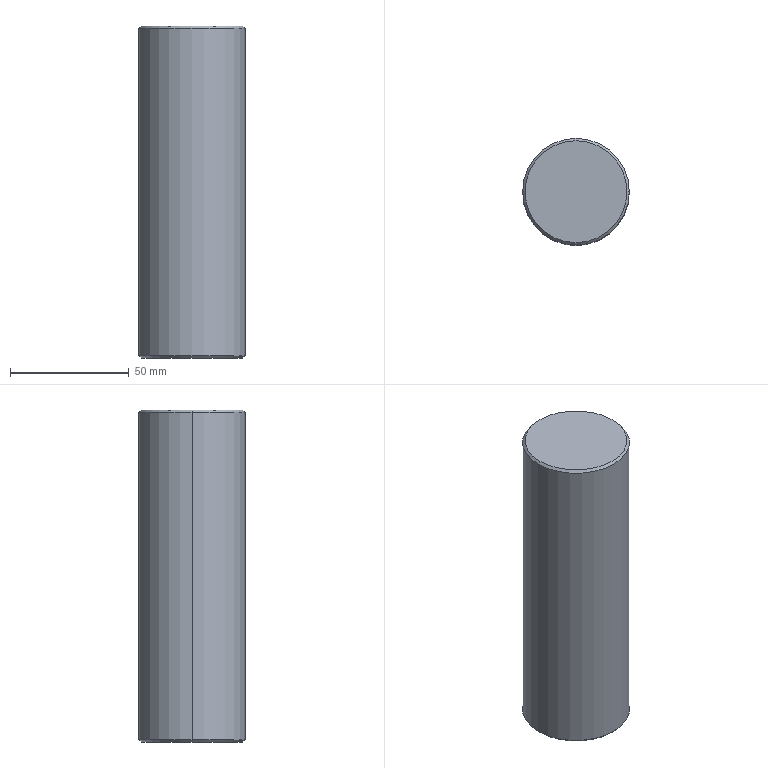Part | Creo | 1 solid | 16 faces | box 45 x 45 x 140 mm | volume 220997 mm3 | cone 8 | cylinder 6 | plane 2 | commonest cylinder face diameters 8.46 x2 10 x2 45 x2
STEP:
#1=CARTESIAN_POINT('',(0.,0.,0.));
#2=DIRECTION('',(0.,0.,1.));
#3=DIRECTION('',(1.,0.,0.));
#4=AXIS2_PLACEMENT_3D('',#1,#2,#3);
#5=CARTESIAN_POINT('',(-29.5,98.,-260.5));
#6=VERTEX_POINT('',#5);
#7=CARTESIAN_POINT('',(-72.5,98.,-260.5));
#8=VERTEX_POINT('',#7);
#9=CARTESIAN_POINT('',(-51.,98.,-260.5));
#10=DIRECTION('',(0.,0.,-1.));
#11=DIRECTION('',(1.,0.,0.));
#12=AXIS2_PLACEMENT_3D('',#9,#10,#11);
#13=CIRCLE('',#12,21.5);
#14=EDGE_CURVE('',#6,#8,#13,.T.);
#15=ORIENTED_EDGE('',*,*,#14,.F.);
#16=CARTESIAN_POINT('',(-51.,98.,-260.5));
#17=DIRECTION('',(0.,0.,-1.));
#18=DIRECTION('',(-1.,0.,0.));
#19=AXIS2_PLACEMENT_3D('',#16,#17,#18);
#20=CIRCLE('',#19,21.5);
#21=EDGE_CURVE('',#8,#6,#20,.T.);
#22=ORIENTED_EDGE('',*,*,#21,.F.);
#23=EDGE_LOOP('',(#15,#22));
#24=FACE_OUTER_BOUND('',#23,.F.);
#25=CARTESIAN_POINT('',(-56.,98.,-260.5));
#26=VERTEX_POINT('',#25);
#27=CARTESIAN_POINT('',(-46.,98.,-260.5));
#28=VERTEX_POINT('',#27);
#29=CARTESIAN_POINT('',(-51.,98.,-260.5));
#30=DIRECTION('',(0.,0.,1.));
#31=DIRECTION('',(-1.,0.,0.));
#32=AXIS2_PLACEMENT_3D('',#29,#30,#31);
#33=CIRCLE('',#32,5.);
#34=EDGE_CURVE('',#26,#28,#33,.T.);
#35=ORIENTED_EDGE('',*,*,#34,.F.);
#36=CARTESIAN_POINT('',(-51.,98.,-260.5));
#37=DIRECTION('',(0.,0.,1.));
#38=DIRECTION('',(1.,0.,0.));
#39=AXIS2_PLACEMENT_3D('',#36,#37,#38);
#40=CIRCLE('',#39,5.);
#41=EDGE_CURVE('',#28,#26,#40,.T.);
#42=ORIENTED_EDGE('',*,*,#41,.F.);
#43=EDGE_LOOP('',(#35,#42));
#44=FACE_BOUND('',#43,.F.);
#45=CARTESIAN_POINT('',(-51.,98.,-260.5));
#46=DIRECTION('',(0.,0.,1.));
#47=DIRECTION('',(1.,0.,0.));
#48=AXIS2_PLACEMENT_3D('',#45,#46,#47);
#49=PLANE('',#48);
#50=ADVANCED_FACE('',(#24,#44),#49,.F.);
#51=ORIENTED_EDGE('',*,*,#14,.T.);
#52=CARTESIAN_POINT('',(-73.5,98.,-259.5));
#53=VERTEX_POINT('',#52);
#54=CARTESIAN_POINT('',(-72.5,98.,-260.5));
#55=DIRECTION('',(-0.7071,0.,0.7071));
#56=VECTOR('',#55,1.414);
#57=LINE('',#54,#56);
#58=EDGE_CURVE('',#8,#53,#57,.T.);
#59=ORIENTED_EDGE('',*,*,#58,.T.);
#60=CARTESIAN_POINT('',(-28.5,98.,-259.5));
#61=VERTEX_POINT('',#60);
#62=CARTESIAN_POINT('',(-51.,98.,-259.5));
#63=DIRECTION('',(0.,0.,-1.));
#64=DIRECTION('',(1.,0.,0.));
#65=AXIS2_PLACEMENT_3D('',#62,#63,#64);
#66=CIRCLE('',#65,22.5);
#67=EDGE_CURVE('',#61,#53,#66,.T.);
#68=ORIENTED_EDGE('',*,*,#67,.F.);
#69=CARTESIAN_POINT('',(-29.5,98.,-260.5));
#70=DIRECTION('',(0.7071,0.,0.7071));
#71=VECTOR('',#70,1.414);
#72=LINE('',#69,#71);
#73=EDGE_CURVE('',#6,#61,#72,.T.);
#74=ORIENTED_EDGE('',*,*,#73,.F.);
#75=EDGE_LOOP('',(#51,#59,#68,#74));
#76=FACE_OUTER_BOUND('',#75,.F.);
#77=CARTESIAN_POINT('',(-51.,98.,-260.));
#78=DIRECTION('',(0.,0.,1.));
#79=DIRECTION('',(1.,0.,0.));
#80=AXIS2_PLACEMENT_3D('',#77,#78,#79);
#81=CONICAL_SURFACE('',#80,22.,45.);
#82=ADVANCED_FACE('',(#76),#81,.T.);
#83=ORIENTED_EDGE('',*,*,#21,.T.);
#84=ORIENTED_EDGE('',*,*,#73,.T.);
#85=CARTESIAN_POINT('',(-51.,98.,-259.5));
#86=DIRECTION('',(0.,0.,-1.));
#87=DIRECTION('',(-1.,0.,0.));
#88=AXIS2_PLACEMENT_3D('',#85,#86,#87);
#89=CIRCLE('',#88,22.5);
#90=EDGE_CURVE('',#53,#61,#89,.T.);
#91=ORIENTED_EDGE('',*,*,#90,.F.);
#92=ORIENTED_EDGE('',*,*,#58,.F.);
#93=EDGE_LOOP('',(#83,#84,#91,#92));
#94=FACE_OUTER_BOUND('',#93,.F.);
#95=CARTESIAN_POINT('',(-51.,98.,-260.));
#96=DIRECTION('',(0.,0.,1.));
#97=DIRECTION('',(1.,0.,0.));
#98=AXIS2_PLACEMENT_3D('',#95,#96,#97);
#99=CONICAL_SURFACE('',#98,22.,45.);
#100=ADVANCED_FACE('',(#94),#99,.T.);
#101=ORIENTED_EDGE('',*,*,#90,.T.);
#102=CARTESIAN_POINT('',(-28.5,98.,-121.5));
#103=VERTEX_POINT('',#102);
#104=CARTESIAN_POINT('',(-28.5,98.,-121.5));
#105=DIRECTION('',(0.,0.,-1.));
#106=VECTOR('',#105,138.);
#107=LINE('',#104,#106);
#108=EDGE_CURVE('',#103,#61,#107,.T.);
#109=ORIENTED_EDGE('',*,*,#108,.F.);
#110=CARTESIAN_POINT('',(-73.5,98.,-121.5));
#111=VERTEX_POINT('',#110);
#112=CARTESIAN_POINT('',(-51.,98.,-121.5));
#113=DIRECTION('',(0.,0.,1.));
#114=DIRECTION('',(1.,0.,0.));
#115=AXIS2_PLACEMENT_3D('',#112,#113,#114);
#116=CIRCLE('',#115,22.5);
#117=EDGE_CURVE('',#103,#111,#116,.T.);
#118=ORIENTED_EDGE('',*,*,#117,.T.);
#119=CARTESIAN_POINT('',(-73.5,98.,-121.5));
#120=DIRECTION('',(0.,0.,-1.));
#121=VECTOR('',#120,138.);
#122=LINE('',#119,#121);
#123=EDGE_CURVE('',#111,#53,#122,.T.);
#124=ORIENTED_EDGE('',*,*,#123,.T.);
#125=EDGE_LOOP('',(#101,#109,#118,#124));
#126=FACE_OUTER_BOUND('',#125,.F.);
#127=CARTESIAN_POINT('',(-51.,98.,-120.5));
#128=DIRECTION('',(0.,0.,-1.));
#129=DIRECTION('',(-1.,0.,0.));
#130=AXIS2_PLACEMENT_3D('',#127,#128,#129);
#131=CYLINDRICAL_SURFACE('',#130,22.5);
#132=ADVANCED_FACE('',(#126),#131,.T.);
#133=ORIENTED_EDGE('',*,*,#67,.T.);
#134=ORIENTED_EDGE('',*,*,#123,.F.);
#135=CARTESIAN_POINT('',(-51.,98.,-121.5));
#136=DIRECTION('',(0.,0.,1.));
#137=DIRECTION('',(-1.,0.,0.));
#138=AXIS2_PLACEMENT_3D('',#135,#136,#137);
#139=CIRCLE('',#138,22.5);
#140=EDGE_CURVE('',#111,#103,#139,.T.);
#141=ORIENTED_EDGE('',*,*,#140,.T.);
#142=ORIENTED_EDGE('',*,*,#108,.T.);
#143=EDGE_LOOP('',(#133,#134,#141,#142));
#144=FACE_OUTER_BOUND('',#143,.F.);
#145=CARTESIAN_POINT('',(-51.,98.,-120.5));
#146=DIRECTION('',(0.,0.,-1.));
#147=DIRECTION('',(-1.,0.,0.));
#148=AXIS2_PLACEMENT_3D('',#145,#146,#147);
#149=CYLINDRICAL_SURFACE('',#148,22.5);
#150=ADVANCED_FACE('',(#144),#149,.T.);
#151=ORIENTED_EDGE('',*,*,#140,.F.);
#152=CARTESIAN_POINT('',(-72.5,98.,-120.5));
#153=VERTEX_POINT('',#152);
#154=CARTESIAN_POINT('',(-72.5,98.,-120.5));
#155=DIRECTION('',(-0.7071,0.,-0.7071));
#156=VECTOR('',#155,1.414);
#157=LINE('',#154,#156);
#158=EDGE_CURVE('',#153,#111,#157,.T.);
#159=ORIENTED_EDGE('',*,*,#158,.F.);
#160=CARTESIAN_POINT('',(-29.5,98.,-120.5));
#161=VERTEX_POINT('',#160);
#162=CARTESIAN_POINT('',(-51.,98.,-120.5));
#163=DIRECTION('',(0.,0.,1.));
#164=DIRECTION('',(-1.,0.,0.));
#165=AXIS2_PLACEMENT_3D('',#162,#163,#164);
#166=CIRCLE('',#165,21.5);
#167=EDGE_CURVE('',#153,#161,#166,.T.);
#168=ORIENTED_EDGE('',*,*,#167,.T.);
#169=CARTESIAN_POINT('',(-29.5,98.,-120.5));
#170=DIRECTION('',(0.7071,0.,-0.7071));
#171=VECTOR('',#170,1.414);
#172=LINE('',#169,#171);
#173=EDGE_CURVE('',#161,#103,#172,.T.);
#174=ORIENTED_EDGE('',*,*,#173,.T.);
#175=EDGE_LOOP('',(#151,#159,#168,#174));
#176=FACE_OUTER_BOUND('',#175,.F.);
#177=CARTESIAN_POINT('',(-51.,98.,-121.));
#178=DIRECTION('',(0.,0.,-1.));
#179=DIRECTION('',(-1.,0.,0.));
#180=AXIS2_PLACEMENT_3D('',#177,#178,#179);
#181=CONICAL_SURFACE('',#180,22.,45.);
#182=ADVANCED_FACE('',(#176),#181,.T.);
#183=ORIENTED_EDGE('',*,*,#117,.F.);
#184=ORIENTED_EDGE('',*,*,#173,.F.);
#185=CARTESIAN_POINT('',(-51.,98.,-120.5));
#186=DIRECTION('',(0.,0.,1.));
#187=DIRECTION('',(1.,0.,0.));
#188=AXIS2_PLACEMENT_3D('',#185,#186,#187);
#189=CIRCLE('',#188,21.5);
#190=EDGE_CURVE('',#161,#153,#189,.T.);
#191=ORIENTED_EDGE('',*,*,#190,.T.);
#192=ORIENTED_EDGE('',*,*,#158,.T.);
#193=EDGE_LOOP('',(#183,#184,#191,#192));
#194=FACE_OUTER_BOUND('',#193,.F.);
#195=CARTESIAN_POINT('',(-51.,98.,-121.));
#196=DIRECTION('',(0.,0.,-1.));
#197=DIRECTION('',(-1.,0.,0.));
#198=AXIS2_PLACEMENT_3D('',#195,#196,#197);
#199=CONICAL_SURFACE('',#198,22.,45.);
#200=ADVANCED_FACE('',(#194),#199,.T.);
#201=ORIENTED_EDGE('',*,*,#190,.F.);
#202=ORIENTED_EDGE('',*,*,#167,.F.);
#203=EDGE_LOOP('',(#201,#202));
#204=FACE_OUTER_BOUND('',#203,.F.);
#205=CARTESIAN_POINT('',(-51.,98.,-120.5));
#206=DIRECTION('',(0.,0.,1.));
#207=DIRECTION('',(1.,0.,0.));
#208=AXIS2_PLACEMENT_3D('',#205,#206,#207);
#209=PLANE('',#208);
#210=ADVANCED_FACE('',(#204),#209,.T.);
#211=CARTESIAN_POINT('',(-46.,98.,-244.5));
#212=VERTEX_POINT('',#211);
#213=CARTESIAN_POINT('',(-56.,98.,-244.5));
#214=VERTEX_POINT('',#213);
#215=CARTESIAN_POINT('',(-51.,98.,-244.5));
#216=DIRECTION('',(0.,0.,-1.));
#217=DIRECTION('',(1.,0.,0.));
#218=AXIS2_PLACEMENT_3D('',#215,#216,#217);
#219=CIRCLE('',#218,5.);
#220=EDGE_CURVE('',#212,#214,#219,.T.);
#221=ORIENTED_EDGE('',*,*,#220,.T.);
#222=CARTESIAN_POINT('',(-56.,98.,-244.5));
#223=DIRECTION('',(0.,0.,-1.));
#224=VECTOR('',#223,16.);
#225=LINE('',#222,#224);
#226=EDGE_CURVE('',#214,#26,#225,.T.);
#227=ORIENTED_EDGE('',*,*,#226,.T.);
#228=ORIENTED_EDGE('',*,*,#34,.T.);
#229=CARTESIAN_POINT('',(-46.,98.,-244.5));
#230=DIRECTION('',(0.,0.,-1.));
#231=VECTOR('',#230,16.);
#232=LINE('',#229,#231);
#233=EDGE_CURVE('',#212,#28,#232,.T.);
#234=ORIENTED_EDGE('',*,*,#233,.F.);
#235=EDGE_LOOP('',(#221,#227,#228,#234));
#236=FACE_OUTER_BOUND('',#235,.F.);
#237=CARTESIAN_POINT('',(-51.,98.,-295.5));
#238=DIRECTION('',(0.,0.,-1.));
#239=DIRECTION('',(-1.,0.,0.));
#240=AXIS2_PLACEMENT_3D('',#237,#238,#239);
#241=CYLINDRICAL_SURFACE('',#240,5.);
#242=ADVANCED_FACE('',(#236),#241,.F.);
#243=CARTESIAN_POINT('',(-55.23,98.,-243.73));
#244=VERTEX_POINT('',#243);
#245=CARTESIAN_POINT('',(-46.77,98.,-243.73));
#246=VERTEX_POINT('',#245);
#247=CARTESIAN_POINT('',(-51.,98.,-243.73));
#248=DIRECTION('',(0.,0.,1.));
#249=DIRECTION('',(-1.,0.,0.));
#250=AXIS2_PLACEMENT_3D('',#247,#248,#249);
#251=CIRCLE('',#250,4.23);
#252=EDGE_CURVE('',#244,#246,#251,.T.);
#253=ORIENTED_EDGE('',*,*,#252,.F.);
#254=CARTESIAN_POINT('',(-55.23,98.,-243.73));
#255=DIRECTION('',(-0.7071,0.,-0.7071));
#256=VECTOR('',#255,1.089);
#257=LINE('',#254,#256);
#258=EDGE_CURVE('',#244,#214,#257,.T.);
#259=ORIENTED_EDGE('',*,*,#258,.T.);
#260=ORIENTED_EDGE('',*,*,#220,.F.);
#261=CARTESIAN_POINT('',(-46.77,98.,-243.73));
#262=DIRECTION('',(0.7071,0.,-0.7071));
#263=VECTOR('',#262,1.089);
#264=LINE('',#261,#263);
#265=EDGE_CURVE('',#246,#212,#264,.T.);
#266=ORIENTED_EDGE('',*,*,#265,.F.);
#267=EDGE_LOOP('',(#253,#259,#260,#266));
#268=FACE_OUTER_BOUND('',#267,.F.);
#269=CARTESIAN_POINT('',(-51.,98.,-244.115));
#270=DIRECTION('',(0.,0.,-1.));
#271=DIRECTION('',(-1.,0.,0.));
#272=AXIS2_PLACEMENT_3D('',#269,#270,#271);
#273=CONICAL_SURFACE('',#272,4.615,45.);
#274=ADVANCED_FACE('',(#268),#273,.F.);
#275=CARTESIAN_POINT('',(-46.77,98.,-240.73));
#276=VERTEX_POINT('',#275);
#277=CARTESIAN_POINT('',(-55.23,98.,-240.73));
#278=VERTEX_POINT('',#277);
#279=CARTESIAN_POINT('',(-51.,98.,-240.73));
#280=DIRECTION('',(0.,0.,-1.));
#281=DIRECTION('',(1.,0.,0.));
#282=AXIS2_PLACEMENT_3D('',#279,#280,#281);
#283=CIRCLE('',#282,4.23);
#284=EDGE_CURVE('',#276,#278,#283,.T.);
#285=ORIENTED_EDGE('',*,*,#284,.T.);
#286=CARTESIAN_POINT('',(-55.23,98.,-240.73));
#287=DIRECTION('',(0.,0.,-1.));
#288=VECTOR('',#287,3.);
#289=LINE('',#286,#288);
#290=EDGE_CURVE('',#278,#244,#289,.T.);
#291=ORIENTED_EDGE('',*,*,#290,.T.);
#292=ORIENTED_EDGE('',*,*,#252,.T.);
#293=CARTESIAN_POINT('',(-46.77,98.,-240.73));
#294=DIRECTION('',(0.,0.,-1.));
#295=VECTOR('',#294,3.);
#296=LINE('',#293,#295);
#297=EDGE_CURVE('',#276,#246,#296,.T.);
#298=ORIENTED_EDGE('',*,*,#297,.F.);
#299=EDGE_LOOP('',(#285,#291,#292,#298));
#300=FACE_OUTER_BOUND('',#299,.F.);
#301=CARTESIAN_POINT('',(-51.,98.,-295.5));
#302=DIRECTION('',(0.,0.,-1.));
#303=DIRECTION('',(-1.,0.,0.));
#304=AXIS2_PLACEMENT_3D('',#301,#302,#303);
#305=CYLINDRICAL_SURFACE('',#304,4.23);
#306=ADVANCED_FACE('',(#300),#305,.F.);
#307=ORIENTED_EDGE('',*,*,#284,.F.);
#308=CARTESIAN_POINT('',(-51.,98.,-238.188));
#309=VERTEX_POINT('',#308);
#310=CARTESIAN_POINT('',(-51.,98.,-238.188));
#311=DIRECTION('',(0.8572,0.,-0.515));
#312=VECTOR('',#311,4.935);
#313=LINE('',#310,#312);
#314=EDGE_CURVE('',#309,#276,#313,.T.);
#315=ORIENTED_EDGE('',*,*,#314,.F.);
#316=CARTESIAN_POINT('',(-51.,98.,-238.188));
#317=DIRECTION('',(-0.8572,0.,-0.515));
#318=VECTOR('',#317,4.935);
#319=LINE('',#316,#318);
#320=EDGE_CURVE('',#309,#278,#319,.T.);
#321=ORIENTED_EDGE('',*,*,#320,.T.);
#322=EDGE_LOOP('',(#307,#315,#321));
#323=FACE_OUTER_BOUND('',#322,.F.);
#324=CARTESIAN_POINT('',(-51.,98.,-239.507));
#325=DIRECTION('',(0.,0.,-1.));
#326=DIRECTION('',(-1.,0.,0.));
#327=AXIS2_PLACEMENT_3D('',#324,#325,#326);
#328=CONICAL_SURFACE('',#327,2.194,59.);
#329=ADVANCED_FACE('',(#323),#328,.F.);
#330=CARTESIAN_POINT('',(-51.,98.,-240.73));
#331=DIRECTION('',(0.,0.,-1.));
#332=DIRECTION('',(-1.,0.,0.));
#333=AXIS2_PLACEMENT_3D('',#330,#331,#332);
#334=CIRCLE('',#333,4.23);
#335=EDGE_CURVE('',#278,#276,#334,.T.);
#336=ORIENTED_EDGE('',*,*,#335,.F.);
#337=ORIENTED_EDGE('',*,*,#320,.F.);
#338=ORIENTED_EDGE('',*,*,#314,.T.);
#339=EDGE_LOOP('',(#336,#337,#338));
#340=FACE_OUTER_BOUND('',#339,.F.);
#341=CARTESIAN_POINT('',(-51.,98.,-239.507));
#342=DIRECTION('',(0.,0.,-1.));
#343=DIRECTION('',(-1.,0.,0.));
#344=AXIS2_PLACEMENT_3D('',#341,#342,#343);
#345=CONICAL_SURFACE('',#344,2.194,59.);
#346=ADVANCED_FACE('',(#340),#345,.F.);
#347=ORIENTED_EDGE('',*,*,#335,.T.);
#348=ORIENTED_EDGE('',*,*,#297,.T.);
#349=CARTESIAN_POINT('',(-51.,98.,-243.73));
#350=DIRECTION('',(0.,0.,1.));
#351=DIRECTION('',(1.,0.,0.));
#352=AXIS2_PLACEMENT_3D('',#349,#350,#351);
#353=CIRCLE('',#352,4.23);
#354=EDGE_CURVE('',#246,#244,#353,.T.);
#355=ORIENTED_EDGE('',*,*,#354,.T.);
#356=ORIENTED_EDGE('',*,*,#290,.F.);
#357=EDGE_LOOP('',(#347,#348,#355,#356));
#358=FACE_OUTER_BOUND('',#357,.F.);
#359=CARTESIAN_POINT('',(-51.,98.,-295.5));
#360=DIRECTION('',(0.,0.,-1.));
#361=DIRECTION('',(-1.,0.,0.));
#362=AXIS2_PLACEMENT_3D('',#359,#360,#361);
#363=CYLINDRICAL_SURFACE('',#362,4.23);
#364=ADVANCED_FACE('',(#358),#363,.F.);
#365=ORIENTED_EDGE('',*,*,#354,.F.);
#366=ORIENTED_EDGE('',*,*,#265,.T.);
#367=CARTESIAN_POINT('',(-51.,98.,-244.5));
#368=DIRECTION('',(0.,0.,-1.));
#369=DIRECTION('',(-1.,0.,0.));
#370=AXIS2_PLACEMENT_3D('',#367,#368,#369);
#371=CIRCLE('',#370,5.);
#372=EDGE_CURVE('',#214,#212,#371,.T.);
#373=ORIENTED_EDGE('',*,*,#372,.F.);
#374=ORIENTED_EDGE('',*,*,#258,.F.);
#375=EDGE_LOOP('',(#365,#366,#373,#374));
#376=FACE_OUTER_BOUND('',#375,.F.);
#377=CARTESIAN_POINT('',(-51.,98.,-244.115));
#378=DIRECTION('',(0.,0.,-1.));
#379=DIRECTION('',(-1.,0.,0.));
#380=AXIS2_PLACEMENT_3D('',#377,#378,#379);
#381=CONICAL_SURFACE('',#380,4.615,45.);
#382=ADVANCED_FACE('',(#376),#381,.F.);
#383=ORIENTED_EDGE('',*,*,#372,.T.);
#384=ORIENTED_EDGE('',*,*,#233,.T.);
#385=ORIENTED_EDGE('',*,*,#41,.T.);
#386=ORIENTED_EDGE('',*,*,#226,.F.);
#387=EDGE_LOOP('',(#383,#384,#385,#386));
#388=FACE_OUTER_BOUND('',#387,.F.);
#389=CARTESIAN_POINT('',(-51.,98.,-295.5));
#390=DIRECTION('',(0.,0.,-1.));
#391=DIRECTION('',(-1.,0.,0.));
#392=AXIS2_PLACEMENT_3D('',#389,#390,#391);
#393=CYLINDRICAL_SURFACE('',#392,5.);
#394=ADVANCED_FACE('',(#388),#393,.F.);
#395=CLOSED_SHELL('',(#50,#82,#100,#132,#150,#182,#200,#210,#242,#274,#306,#329,#346,#364,#382,#394));
#396=MANIFOLD_SOLID_BREP('',#395);
#397=(LENGTH_UNIT()NAMED_UNIT(*)SI_UNIT(.MILLI.,.METRE.));
#398=UNCERTAINTY_MEASURE_WITH_UNIT(LENGTH_MEASURE(0.01538),#397,'','');
#399=(NAMED_UNIT(*)PLANE_ANGLE_UNIT()SI_UNIT($,.RADIAN.));
#400=PLANE_ANGLE_MEASURE_WITH_UNIT(PLANE_ANGLE_MEASURE(0.01745),#399);
#401=(CONVERSION_BASED_UNIT('DEGREE',#400)NAMED_UNIT(*)PLANE_ANGLE_UNIT());
#402=(NAMED_UNIT(*)SI_UNIT($,.STERADIAN.)SOLID_ANGLE_UNIT());
#403=(GEOMETRIC_REPRESENTATION_CONTEXT(3)GLOBAL_UNCERTAINTY_ASSIGNED_CONTEXT((#398))GLOBAL_UNIT_ASSIGNED_CONTEXT((#397,#401,#402))REPRESENTATION_CONTEXT('',''));
#404=ADVANCED_BREP_SHAPE_REPRESENTATION('',(#4,#396),#403);